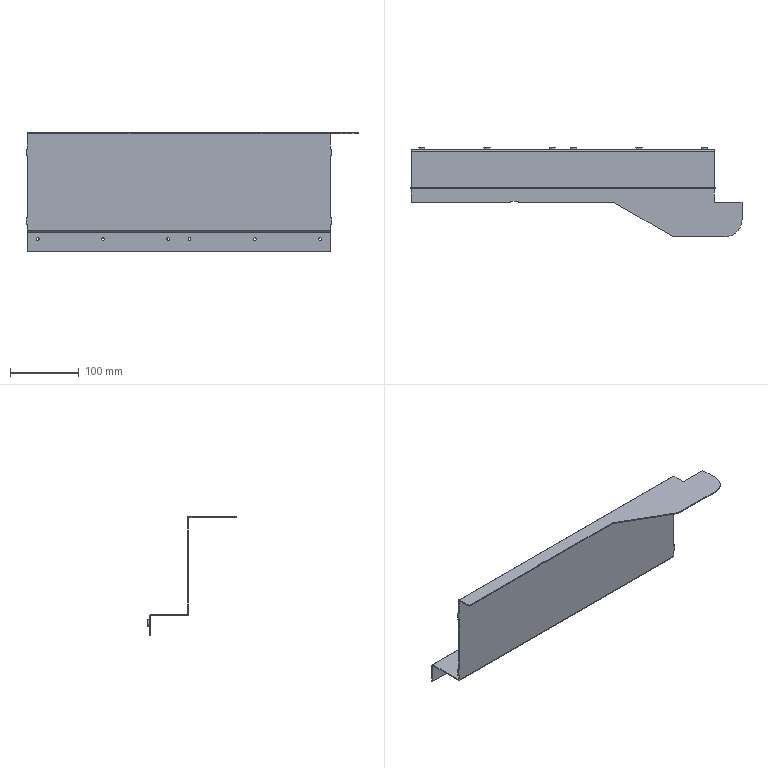Part | STEP file | FHD-021-001-J rack welded part J | 1 solid | 61 faces | box 482.9 x 130.5 x 173 mm | volume 174985 mm3 | plane 42 | cylinder 19 | commonest cylinder face diameters 4.2 x6 9.2 x6 0.4 x3 3.4 x3 50 x1